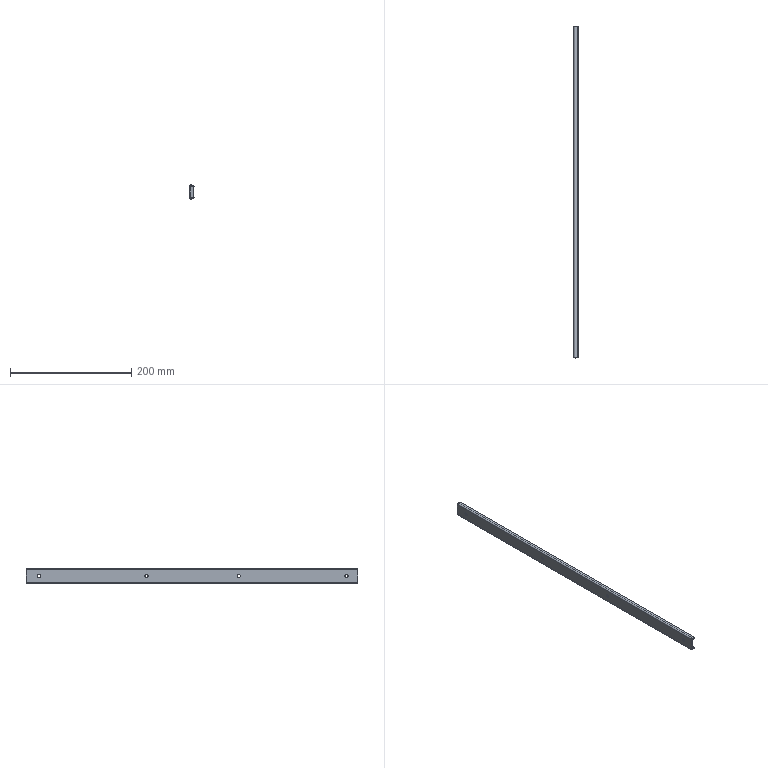Part | NX | features SLIDER_5003_009_C-SRH51Y22 2 | 1 solid | 39 faces | box 7 x 548.5 x 23.6 mm | volume 29924 mm3 | plane 20 | cylinder 19 | commonest cylinder face diameters 4.5 x8 0.4 x2 2 x2 3.6 x2 4.8 x2 8 x2
STEP:
#1=CARTESIAN_POINT('',(193.825,-253.,-88.75));
#2=VERTEX_POINT('',#1);
#3=CARTESIAN_POINT('',(193.825,-253.,-84.25));
#4=VERTEX_POINT('',#3);
#5=CARTESIAN_POINT('',(193.825,-253.,-86.5));
#6=DIRECTION('',(1.,0.,0.));
#7=DIRECTION('',(0.,0.,-1.));
#8=AXIS2_PLACEMENT_3D('',#5,#6,#7);
#9=CIRCLE('',#8,2.25);
#10=EDGE_CURVE('',#2,#4,#9,.F.);
#11=ORIENTED_EDGE('',*,*,#10,.F.);
#12=CARTESIAN_POINT('',(193.825,-252.2,-88.75));
#13=VERTEX_POINT('',#12);
#14=CARTESIAN_POINT('',(193.825,99.,-88.75));
#15=DIRECTION('',(0.,-1.,0.));
#16=VECTOR('',#15,1000.);
#17=LINE('',#14,#16);
#18=EDGE_CURVE('',#13,#2,#17,.T.);
#19=ORIENTED_EDGE('',*,*,#18,.F.);
#20=CARTESIAN_POINT('',(193.825,-252.2,-84.25));
#21=VERTEX_POINT('',#20);
#22=CARTESIAN_POINT('',(193.825,-252.2,-86.5));
#23=DIRECTION('',(1.,0.,0.));
#24=DIRECTION('',(0.,0.,-1.));
#25=AXIS2_PLACEMENT_3D('',#22,#23,#24);
#26=CIRCLE('',#25,2.25);
#27=EDGE_CURVE('',#21,#13,#26,.F.);
#28=ORIENTED_EDGE('',*,*,#27,.F.);
#29=CARTESIAN_POINT('',(193.825,99.,-84.25));
#30=DIRECTION('',(0.,1.,0.));
#31=VECTOR('',#30,1000.);
#32=LINE('',#29,#31);
#33=EDGE_CURVE('',#4,#21,#32,.T.);
#34=ORIENTED_EDGE('',*,*,#33,.F.);
#35=EDGE_LOOP('',(#11,#19,#28,#34));
#36=FACE_BOUND('',#35,.T.);
#37=CARTESIAN_POINT('',(193.825,-430.8,-88.75));
#38=VERTEX_POINT('',#37);
#39=CARTESIAN_POINT('',(193.825,-430.8,-84.25));
#40=VERTEX_POINT('',#39);
#41=CARTESIAN_POINT('',(193.825,-430.8,-86.5));
#42=DIRECTION('',(1.,0.,0.));
#43=DIRECTION('',(0.,0.,-1.));
#44=AXIS2_PLACEMENT_3D('',#41,#42,#43);
#45=CIRCLE('',#44,2.25);
#46=EDGE_CURVE('',#38,#40,#45,.F.);
#47=ORIENTED_EDGE('',*,*,#46,.F.);
#48=CARTESIAN_POINT('',(193.825,-430.,-88.75));
#49=VERTEX_POINT('',#48);
#50=CARTESIAN_POINT('',(193.825,99.,-88.75));
#51=DIRECTION('',(0.,-1.,0.));
#52=VECTOR('',#51,1000.);
#53=LINE('',#50,#52);
#54=EDGE_CURVE('',#49,#38,#53,.T.);
#55=ORIENTED_EDGE('',*,*,#54,.F.);
#56=CARTESIAN_POINT('',(193.825,-430.,-84.25));
#57=VERTEX_POINT('',#56);
#58=CARTESIAN_POINT('',(193.825,-430.,-86.5));
#59=DIRECTION('',(1.,0.,0.));
#60=DIRECTION('',(0.,0.,-1.));
#61=AXIS2_PLACEMENT_3D('',#58,#59,#60);
#62=CIRCLE('',#61,2.25);
#63=EDGE_CURVE('',#57,#49,#62,.F.);
#64=ORIENTED_EDGE('',*,*,#63,.F.);
#65=CARTESIAN_POINT('',(193.825,99.,-84.25));
#66=DIRECTION('',(0.,1.,0.));
#67=VECTOR('',#66,1000.);
#68=LINE('',#65,#67);
#69=EDGE_CURVE('',#40,#57,#68,.T.);
#70=ORIENTED_EDGE('',*,*,#69,.F.);
#71=EDGE_LOOP('',(#47,#55,#64,#70));
#72=FACE_BOUND('',#71,.T.);
#73=CARTESIAN_POINT('',(193.825,97.4,-77.5));
#74=VERTEX_POINT('',#73);
#75=CARTESIAN_POINT('',(193.825,97.4,-76.5));
#76=VERTEX_POINT('',#75);
#77=CARTESIAN_POINT('',(193.825,97.4,-98.3));
#78=DIRECTION('',(0.,0.,1.));
#79=VECTOR('',#78,1000.);
#80=LINE('',#77,#79);
#81=EDGE_CURVE('',#74,#76,#80,.T.);
#82=ORIENTED_EDGE('',*,*,#81,.F.);
#83=CARTESIAN_POINT('',(193.825,97.4,-95.5));
#84=VERTEX_POINT('',#83);
#85=CARTESIAN_POINT('',(193.825,97.4,-96.5));
#86=DIRECTION('',(0.,0.,1.));
#87=VECTOR('',#86,1000.);
#88=LINE('',#85,#87);
#89=EDGE_CURVE('',#74,#84,#88,.F.);
#90=ORIENTED_EDGE('',*,*,#89,.T.);
#91=CARTESIAN_POINT('',(193.825,97.4,-96.5));
#92=VERTEX_POINT('',#91);
#93=CARTESIAN_POINT('',(193.825,97.4,-98.3));
#94=DIRECTION('',(0.,0.,1.));
#95=VECTOR('',#94,1000.);
#96=LINE('',#93,#95);
#97=EDGE_CURVE('',#92,#84,#96,.T.);
#98=ORIENTED_EDGE('',*,*,#97,.F.);
#99=CARTESIAN_POINT('',(193.825,-449.5,-96.5));
#100=VERTEX_POINT('',#99);
#101=CARTESIAN_POINT('',(193.825,99.,-96.5));
#102=DIRECTION('',(0.,-1.,0.));
#103=VECTOR('',#102,1000.);
#104=LINE('',#101,#103);
#105=EDGE_CURVE('',#92,#100,#104,.T.);
#106=ORIENTED_EDGE('',*,*,#105,.T.);
#107=CARTESIAN_POINT('',(193.825,-449.5,-76.5));
#108=VERTEX_POINT('',#107);
#109=CARTESIAN_POINT('',(193.825,-449.5,-96.5));
#110=DIRECTION('',(0.,0.,1.));
#111=VECTOR('',#110,1000.);
#112=LINE('',#109,#111);
#113=EDGE_CURVE('',#100,#108,#112,.T.);
#114=ORIENTED_EDGE('',*,*,#113,.T.);
#115=CARTESIAN_POINT('',(193.825,99.,-76.5));
#116=DIRECTION('',(0.,-1.,0.));
#117=VECTOR('',#116,1000.);
#118=LINE('',#115,#117);
#119=EDGE_CURVE('',#76,#108,#118,.T.);
#120=ORIENTED_EDGE('',*,*,#119,.F.);
#121=EDGE_LOOP('',(#82,#90,#98,#106,#114,#120));
#122=FACE_BOUND('',#121,.T.);
#123=CARTESIAN_POINT('',(193.825,78.,-84.25));
#124=VERTEX_POINT('',#123);
#125=CARTESIAN_POINT('',(193.825,78.,-88.75));
#126=VERTEX_POINT('',#125);
#127=CARTESIAN_POINT('',(193.825,78.,-86.5));
#128=DIRECTION('',(1.,0.,0.));
#129=DIRECTION('',(0.,0.,-1.));
#130=AXIS2_PLACEMENT_3D('',#127,#128,#129);
#131=CIRCLE('',#130,2.25);
#132=EDGE_CURVE('',#124,#126,#131,.F.);
#133=ORIENTED_EDGE('',*,*,#132,.F.);
#134=CARTESIAN_POINT('',(193.825,77.2,-84.25));
#135=VERTEX_POINT('',#134);
#136=CARTESIAN_POINT('',(193.825,99.,-84.25));
#137=DIRECTION('',(0.,1.,0.));
#138=VECTOR('',#137,1000.);
#139=LINE('',#136,#138);
#140=EDGE_CURVE('',#135,#124,#139,.T.);
#141=ORIENTED_EDGE('',*,*,#140,.F.);
#142=CARTESIAN_POINT('',(193.825,77.2,-88.75));
#143=VERTEX_POINT('',#142);
#144=CARTESIAN_POINT('',(193.825,77.2,-86.5));
#145=DIRECTION('',(1.,0.,0.));
#146=DIRECTION('',(0.,0.,-1.));
#147=AXIS2_PLACEMENT_3D('',#144,#145,#146);
#148=CIRCLE('',#147,2.25);
#149=EDGE_CURVE('',#143,#135,#148,.F.);
#150=ORIENTED_EDGE('',*,*,#149,.F.);
#151=CARTESIAN_POINT('',(193.825,99.,-88.75));
#152=DIRECTION('',(0.,-1.,0.));
#153=VECTOR('',#152,1000.);
#154=LINE('',#151,#153);
#155=EDGE_CURVE('',#126,#143,#154,.T.);
#156=ORIENTED_EDGE('',*,*,#155,.F.);
#157=EDGE_LOOP('',(#133,#141,#150,#156));
#158=FACE_BOUND('',#157,.T.);
#159=CARTESIAN_POINT('',(193.825,-100.6,-88.75));
#160=VERTEX_POINT('',#159);
#161=CARTESIAN_POINT('',(193.825,-100.6,-84.25));
#162=VERTEX_POINT('',#161);
#163=CARTESIAN_POINT('',(193.825,-100.6,-86.5));
#164=DIRECTION('',(1.,0.,0.));
#165=DIRECTION('',(0.,0.,-1.));
#166=AXIS2_PLACEMENT_3D('',#163,#164,#165);
#167=CIRCLE('',#166,2.25);
#168=EDGE_CURVE('',#160,#162,#167,.F.);
#169=ORIENTED_EDGE('',*,*,#168,.F.);
#170=CARTESIAN_POINT('',(193.825,-99.8,-88.75));
#171=VERTEX_POINT('',#170);
#172=CARTESIAN_POINT('',(193.825,99.,-88.75));
#173=DIRECTION('',(0.,-1.,0.));
#174=VECTOR('',#173,1000.);
#175=LINE('',#172,#174);
#176=EDGE_CURVE('',#171,#160,#175,.T.);
#177=ORIENTED_EDGE('',*,*,#176,.F.);
#178=CARTESIAN_POINT('',(193.825,-99.8,-84.25));
#179=VERTEX_POINT('',#178);
#180=CARTESIAN_POINT('',(193.825,-99.8,-86.5));
#181=DIRECTION('',(1.,0.,0.));
#182=DIRECTION('',(0.,0.,-1.));
#183=AXIS2_PLACEMENT_3D('',#180,#181,#182);
#184=CIRCLE('',#183,2.25);
#185=EDGE_CURVE('',#179,#171,#184,.F.);
#186=ORIENTED_EDGE('',*,*,#185,.F.);
#187=CARTESIAN_POINT('',(193.825,99.,-84.25));
#188=DIRECTION('',(0.,1.,0.));
#189=VECTOR('',#188,1000.);
#190=LINE('',#187,#189);
#191=EDGE_CURVE('',#162,#179,#190,.T.);
#192=ORIENTED_EDGE('',*,*,#191,.F.);
#193=EDGE_LOOP('',(#169,#177,#186,#192));
#194=FACE_BOUND('',#193,.T.);
#195=CARTESIAN_POINT('',(193.825,99.,-96.5));
#196=DIRECTION('',(1.,0.,0.));
#197=DIRECTION('',(0.,0.,-1.));
#198=AXIS2_PLACEMENT_3D('',#195,#196,#197);
#199=PLANE('',#198);
#200=ADVANCED_FACE('',(#36,#72,#122,#158,#194),#199,.F.);
#201=CARTESIAN_POINT('',(195.425,-253.,-88.75));
#202=VERTEX_POINT('',#201);
#203=CARTESIAN_POINT('',(195.425,-253.,-84.25));
#204=VERTEX_POINT('',#203);
#205=CARTESIAN_POINT('',(195.425,-253.,-86.5));
#206=DIRECTION('',(-1.,0.,0.));
#207=DIRECTION('',(0.,1.,0.));
#208=AXIS2_PLACEMENT_3D('',#205,#206,#207);
#209=CIRCLE('',#208,2.25);
#210=EDGE_CURVE('',#202,#204,#209,.T.);
#211=ORIENTED_EDGE('',*,*,#210,.T.);
#212=CARTESIAN_POINT('',(195.425,-252.2,-84.25));
#213=VERTEX_POINT('',#212);
#214=CARTESIAN_POINT('',(195.425,-253.,-84.25));
#215=DIRECTION('',(0.,1.,0.));
#216=VECTOR('',#215,1000.);
#217=LINE('',#214,#216);
#218=EDGE_CURVE('',#204,#213,#217,.T.);
#219=ORIENTED_EDGE('',*,*,#218,.T.);
#220=CARTESIAN_POINT('',(195.425,-252.2,-88.75));
#221=VERTEX_POINT('',#220);
#222=CARTESIAN_POINT('',(195.425,-252.2,-86.5));
#223=DIRECTION('',(-1.,0.,0.));
#224=DIRECTION('',(0.,1.,0.));
#225=AXIS2_PLACEMENT_3D('',#222,#223,#224);
#226=CIRCLE('',#225,2.25);
#227=EDGE_CURVE('',#213,#221,#226,.T.);
#228=ORIENTED_EDGE('',*,*,#227,.T.);
#229=CARTESIAN_POINT('',(195.425,-253.,-88.75));
#230=DIRECTION('',(0.,-1.,0.));
#231=VECTOR('',#230,1000.);
#232=LINE('',#229,#231);
#233=EDGE_CURVE('',#221,#202,#232,.T.);
#234=ORIENTED_EDGE('',*,*,#233,.T.);
#235=EDGE_LOOP('',(#211,#219,#228,#234));
#236=FACE_BOUND('',#235,.T.);
#237=CARTESIAN_POINT('',(195.425,-430.8,-88.75));
#238=VERTEX_POINT('',#237);
#239=CARTESIAN_POINT('',(195.425,-430.8,-84.25));
#240=VERTEX_POINT('',#239);
#241=CARTESIAN_POINT('',(195.425,-430.8,-86.5));
#242=DIRECTION('',(-1.,0.,0.));
#243=DIRECTION('',(0.,1.,0.));
#244=AXIS2_PLACEMENT_3D('',#241,#242,#243);
#245=CIRCLE('',#244,2.25);
#246=EDGE_CURVE('',#238,#240,#245,.T.);
#247=ORIENTED_EDGE('',*,*,#246,.T.);
#248=CARTESIAN_POINT('',(195.425,-430.,-84.25));
#249=VERTEX_POINT('',#248);
#250=CARTESIAN_POINT('',(195.425,-430.8,-84.25));
#251=DIRECTION('',(0.,1.,0.));
#252=VECTOR('',#251,1000.);
#253=LINE('',#250,#252);
#254=EDGE_CURVE('',#240,#249,#253,.T.);
#255=ORIENTED_EDGE('',*,*,#254,.T.);
#256=CARTESIAN_POINT('',(195.425,-430.,-88.75));
#257=VERTEX_POINT('',#256);
#258=CARTESIAN_POINT('',(195.425,-430.,-86.5));
#259=DIRECTION('',(-1.,0.,0.));
#260=DIRECTION('',(0.,1.,0.));
#261=AXIS2_PLACEMENT_3D('',#258,#259,#260);
#262=CIRCLE('',#261,2.25);
#263=EDGE_CURVE('',#249,#257,#262,.T.);
#264=ORIENTED_EDGE('',*,*,#263,.T.);
#265=CARTESIAN_POINT('',(195.425,-430.8,-88.75));
#266=DIRECTION('',(0.,-1.,0.));
#267=VECTOR('',#266,1000.);
#268=LINE('',#265,#267);
#269=EDGE_CURVE('',#257,#238,#268,.T.);
#270=ORIENTED_EDGE('',*,*,#269,.T.);
#271=EDGE_LOOP('',(#247,#255,#264,#270));
#272=FACE_BOUND('',#271,.T.);
#273=CARTESIAN_POINT('',(195.425,97.4,-96.5));
#274=VERTEX_POINT('',#273);
#275=CARTESIAN_POINT('',(195.425,-449.5,-96.5));
#276=VERTEX_POINT('',#275);
#277=CARTESIAN_POINT('',(195.425,99.,-96.5));
#278=DIRECTION('',(0.,-1.,0.));
#279=VECTOR('',#278,1000.);
#280=LINE('',#277,#279);
#281=EDGE_CURVE('',#274,#276,#280,.T.);
#282=ORIENTED_EDGE('',*,*,#281,.F.);
#283=CARTESIAN_POINT('',(195.425,97.4,-95.5));
#284=VERTEX_POINT('',#283);
#285=CARTESIAN_POINT('',(195.425,97.4,-96.5));
#286=DIRECTION('',(0.,0.,1.));
#287=VECTOR('',#286,1000.);
#288=LINE('',#285,#287);
#289=EDGE_CURVE('',#274,#284,#288,.T.);
#290=ORIENTED_EDGE('',*,*,#289,.T.);
#291=CARTESIAN_POINT('',(195.425,97.4,-77.5));
#292=VERTEX_POINT('',#291);
#293=CARTESIAN_POINT('',(195.425,97.4,-96.5));
#294=DIRECTION('',(0.,0.,1.));
#295=VECTOR('',#294,1000.);
#296=LINE('',#293,#295);
#297=EDGE_CURVE('',#284,#292,#296,.T.);
#298=ORIENTED_EDGE('',*,*,#297,.T.);
#299=CARTESIAN_POINT('',(195.425,97.4,-76.5));
#300=VERTEX_POINT('',#299);
#301=CARTESIAN_POINT('',(195.425,97.4,-96.5));
#302=DIRECTION('',(0.,0.,1.));
#303=VECTOR('',#302,1000.);
#304=LINE('',#301,#303);
#305=EDGE_CURVE('',#292,#300,#304,.T.);
#306=ORIENTED_EDGE('',*,*,#305,.T.);
#307=CARTESIAN_POINT('',(195.425,-449.5,-76.5));
#308=VERTEX_POINT('',#307);
#309=CARTESIAN_POINT('',(195.425,99.,-76.5));
#310=DIRECTION('',(0.,-1.,0.));
#311=VECTOR('',#310,1000.);
#312=LINE('',#309,#311);
#313=EDGE_CURVE('',#300,#308,#312,.T.);
#314=ORIENTED_EDGE('',*,*,#313,.T.);
#315=CARTESIAN_POINT('',(195.425,-449.5,-96.5));
#316=DIRECTION('',(0.,0.,-1.));
#317=VECTOR('',#316,1000.);
#318=LINE('',#315,#317);
#319=EDGE_CURVE('',#308,#276,#318,.T.);
#320=ORIENTED_EDGE('',*,*,#319,.T.);
#321=EDGE_LOOP('',(#282,#290,#298,#306,#314,#320));
#322=FACE_BOUND('',#321,.T.);
#323=CARTESIAN_POINT('',(195.425,78.,-84.25));
#324=VERTEX_POINT('',#323);
#325=CARTESIAN_POINT('',(195.425,78.,-88.75));
#326=VERTEX_POINT('',#325);
#327=CARTESIAN_POINT('',(195.425,78.,-86.5));
#328=DIRECTION('',(-1.,0.,0.));
#329=DIRECTION('',(0.,1.,0.));
#330=AXIS2_PLACEMENT_3D('',#327,#328,#329);
#331=CIRCLE('',#330,2.25);
#332=EDGE_CURVE('',#324,#326,#331,.T.);
#333=ORIENTED_EDGE('',*,*,#332,.T.);
#334=CARTESIAN_POINT('',(195.425,77.2,-88.75));
#335=VERTEX_POINT('',#334);
#336=CARTESIAN_POINT('',(195.425,77.2,-88.75));
#337=DIRECTION('',(0.,-1.,0.));
#338=VECTOR('',#337,1000.);
#339=LINE('',#336,#338);
#340=EDGE_CURVE('',#326,#335,#339,.T.);
#341=ORIENTED_EDGE('',*,*,#340,.T.);
#342=CARTESIAN_POINT('',(195.425,77.2,-84.25));
#343=VERTEX_POINT('',#342);
#344=CARTESIAN_POINT('',(195.425,77.2,-86.5));
#345=DIRECTION('',(-1.,0.,0.));
#346=DIRECTION('',(0.,1.,0.));
#347=AXIS2_PLACEMENT_3D('',#344,#345,#346);
#348=CIRCLE('',#347,2.25);
#349=EDGE_CURVE('',#335,#343,#348,.T.);
#350=ORIENTED_EDGE('',*,*,#349,.T.);
#351=CARTESIAN_POINT('',(195.425,77.2,-84.25));
#352=DIRECTION('',(0.,1.,0.));
#353=VECTOR('',#352,1000.);
#354=LINE('',#351,#353);
#355=EDGE_CURVE('',#343,#324,#354,.T.);
#356=ORIENTED_EDGE('',*,*,#355,.T.);
#357=EDGE_LOOP('',(#333,#341,#350,#356));
#358=FACE_BOUND('',#357,.T.);
#359=CARTESIAN_POINT('',(195.425,-100.6,-88.75));
#360=VERTEX_POINT('',#359);
#361=CARTESIAN_POINT('',(195.425,-100.6,-84.25));
#362=VERTEX_POINT('',#361);
#363=CARTESIAN_POINT('',(195.425,-100.6,-86.5));
#364=DIRECTION('',(-1.,0.,0.));
#365=DIRECTION('',(0.,1.,0.));
#366=AXIS2_PLACEMENT_3D('',#363,#364,#365);
#367=CIRCLE('',#366,2.25);
#368=EDGE_CURVE('',#360,#362,#367,.T.);
#369=ORIENTED_EDGE('',*,*,#368,.T.);
#370=CARTESIAN_POINT('',(195.425,-99.8,-84.25));
#371=VERTEX_POINT('',#370);
#372=CARTESIAN_POINT('',(195.425,-100.6,-84.25));
#373=DIRECTION('',(0.,1.,0.));
#374=VECTOR('',#373,1000.);
#375=LINE('',#372,#374);
#376=EDGE_CURVE('',#362,#371,#375,.T.);
#377=ORIENTED_EDGE('',*,*,#376,.T.);
#378=CARTESIAN_POINT('',(195.425,-99.8,-88.75));
#379=VERTEX_POINT('',#378);
#380=CARTESIAN_POINT('',(195.425,-99.8,-86.5));
#381=DIRECTION('',(-1.,0.,0.));
#382=DIRECTION('',(0.,1.,0.));
#383=AXIS2_PLACEMENT_3D('',#380,#381,#382);
#384=CIRCLE('',#383,2.25);
#385=EDGE_CURVE('',#371,#379,#384,.T.);
#386=ORIENTED_EDGE('',*,*,#385,.T.);
#387=CARTESIAN_POINT('',(195.425,-100.6,-88.75));
#388=DIRECTION('',(0.,-1.,0.));
#389=VECTOR('',#388,1000.);
#390=LINE('',#387,#389);
#391=EDGE_CURVE('',#379,#360,#390,.T.);
#392=ORIENTED_EDGE('',*,*,#391,.T.);
#393=EDGE_LOOP('',(#369,#377,#386,#392));
#394=FACE_BOUND('',#393,.T.);
#395=CARTESIAN_POINT('',(195.425,99.,-96.5));
#396=DIRECTION('',(-1.,0.,0.));
#397=DIRECTION('',(0.,0.,1.));
#398=AXIS2_PLACEMENT_3D('',#395,#396,#397);
#399=PLANE('',#398);
#400=ADVANCED_FACE('',(#236,#272,#322,#358,#394),#399,.F.);
#401=CARTESIAN_POINT('',(198.325,97.4,-95.5));
#402=VERTEX_POINT('',#401);
#403=CARTESIAN_POINT('',(197.931,97.4,-95.5));
#404=VERTEX_POINT('',#403);
#405=CARTESIAN_POINT('',(199.325,97.4,-95.5));
#406=DIRECTION('',(-1.,0.,0.));
#407=VECTOR('',#406,1000.);
#408=LINE('',#405,#407);
#409=EDGE_CURVE('',#402,#404,#408,.T.);
#410=ORIENTED_EDGE('',*,*,#409,.F.);
#411=CARTESIAN_POINT('',(198.667,97.4,-95.44));
#412=VERTEX_POINT('',#411);
#413=CARTESIAN_POINT('',(198.325,97.4,-94.5));
#414=DIRECTION('',(0.,-1.,0.));
#415=DIRECTION('',(-1.,0.,0.));
#416=AXIS2_PLACEMENT_3D('',#413,#414,#415);
#417=CIRCLE('',#416,1.);
#418=EDGE_CURVE('',#402,#412,#417,.T.);
#419=ORIENTED_EDGE('',*,*,#418,.T.);
#420=CARTESIAN_POINT('',(200.825,97.4,-96.099));
#421=VERTEX_POINT('',#420);
#422=CARTESIAN_POINT('',(198.625,97.4,-99.439));
#423=DIRECTION('',(0.,-1.,0.));
#424=DIRECTION('',(-1.,0.,0.));
#425=AXIS2_PLACEMENT_3D('',#422,#423,#424);
#426=CIRCLE('',#425,4.);
#427=EDGE_CURVE('',#421,#412,#426,.T.);
#428=ORIENTED_EDGE('',*,*,#427,.F.);
#429=CARTESIAN_POINT('',(200.425,97.4,-97.852));
#430=VERTEX_POINT('',#429);
#431=CARTESIAN_POINT('',(200.425,97.4,-97.852));
#432=DIRECTION('',(0.2224,0.,0.9749));
#433=VECTOR('',#432,1000.);
#434=LINE('',#431,#433);
#435=EDGE_CURVE('',#430,#421,#434,.T.);
#436=ORIENTED_EDGE('',*,*,#435,.F.);
#437=CARTESIAN_POINT('',(196.911,97.4,-97.76));
#438=VERTEX_POINT('',#437);
#439=CARTESIAN_POINT('',(198.625,97.4,-99.439));
#440=DIRECTION('',(0.,-1.,0.));
#441=DIRECTION('',(-1.,0.,0.));
#442=AXIS2_PLACEMENT_3D('',#439,#440,#441);
#443=CIRCLE('',#442,2.4);
#444=EDGE_CURVE('',#438,#430,#443,.F.);
#445=ORIENTED_EDGE('',*,*,#444,.F.);
#446=CARTESIAN_POINT('',(195.625,97.4,-96.5));
#447=DIRECTION('',(0.,-1.,0.));
#448=DIRECTION('',(-1.,0.,0.));
#449=AXIS2_PLACEMENT_3D('',#446,#447,#448);
#450=CIRCLE('',#449,1.8);
#451=EDGE_CURVE('',#92,#438,#450,.T.);
#452=ORIENTED_EDGE('',*,*,#451,.F.);
#453=ORIENTED_EDGE('',*,*,#97,.T.);
#454=CARTESIAN_POINT('',(199.325,97.4,-95.5));
#455=DIRECTION('',(-1.,0.,0.));
#456=VECTOR('',#455,1000.);
#457=LINE('',#454,#456);
#458=EDGE_CURVE('',#284,#84,#457,.T.);
#459=ORIENTED_EDGE('',*,*,#458,.F.);
#460=ORIENTED_EDGE('',*,*,#289,.F.);
#461=CARTESIAN_POINT('',(195.768,97.4,-96.64));
#462=VERTEX_POINT('',#461);
#463=CARTESIAN_POINT('',(195.625,97.4,-96.5));
#464=DIRECTION('',(0.,-1.,0.));
#465=DIRECTION('',(-1.,0.,0.));
#466=AXIS2_PLACEMENT_3D('',#463,#464,#465);
#467=CIRCLE('',#466,0.2);
#468=EDGE_CURVE('',#462,#274,#467,.F.);
#469=ORIENTED_EDGE('',*,*,#468,.F.);
#470=CARTESIAN_POINT('',(198.625,97.4,-99.439));
#471=DIRECTION('',(0.,-1.,0.));
#472=DIRECTION('',(-1.,0.,0.));
#473=AXIS2_PLACEMENT_3D('',#470,#471,#472);
#474=CIRCLE('',#473,4.);
#475=EDGE_CURVE('',#404,#462,#474,.T.);
#476=ORIENTED_EDGE('',*,*,#475,.F.);
#477=EDGE_LOOP('',(#410,#419,#428,#436,#445,#452,#453,#459,#460,#469,#476));
#478=FACE_BOUND('',#477,.T.);
#479=CARTESIAN_POINT('',(200.825,97.4,-98.3));
#480=DIRECTION('',(0.,-1.,0.));
#481=DIRECTION('',(-1.,0.,0.));
#482=AXIS2_PLACEMENT_3D('',#479,#480,#481);
#483=PLANE('',#482);
#484=ADVANCED_FACE('',(#478),#483,.F.);
#485=ORIENTED_EDGE('',*,*,#105,.F.);
#486=ORIENTED_EDGE('',*,*,#451,.T.);
#487=CARTESIAN_POINT('',(196.911,-449.5,-97.76));
#488=VERTEX_POINT('',#487);
#489=CARTESIAN_POINT('',(196.911,99.,-97.76));
#490=DIRECTION('',(0.,-1.,0.));
#491=VECTOR('',#490,1000.);
#492=LINE('',#489,#491);
#493=EDGE_CURVE('',#438,#488,#492,.T.);
#494=ORIENTED_EDGE('',*,*,#493,.T.);
#495=CARTESIAN_POINT('',(195.625,-449.5,-96.5));
#496=DIRECTION('',(0.,1.,0.));
#497=DIRECTION('',(-1.,0.,0.));
#498=AXIS2_PLACEMENT_3D('',#495,#496,#497);
#499=CIRCLE('',#498,1.8);
#500=EDGE_CURVE('',#488,#100,#499,.T.);
#501=ORIENTED_EDGE('',*,*,#500,.T.);
#502=EDGE_LOOP('',(#485,#486,#494,#501));
#503=FACE_BOUND('',#502,.T.);
#504=CARTESIAN_POINT('',(195.625,99.,-96.5));
#505=DIRECTION('',(0.,-1.,0.));
#506=DIRECTION('',(-1.,0.,0.));
#507=AXIS2_PLACEMENT_3D('',#504,#505,#506);
#508=CYLINDRICAL_SURFACE('',#507,1.8);
#509=ADVANCED_FACE('',(#503),#508,.T.);
#510=CARTESIAN_POINT('',(196.911,97.4,-75.24));
#511=VERTEX_POINT('',#510);
#512=CARTESIAN_POINT('',(196.911,-449.5,-75.24));
#513=VERTEX_POINT('',#512);
#514=CARTESIAN_POINT('',(196.911,99.,-75.24));
#515=DIRECTION('',(0.,-1.,0.));
#516=VECTOR('',#515,1000.);
#517=LINE('',#514,#516);
#518=EDGE_CURVE('',#511,#513,#517,.T.);
#519=ORIENTED_EDGE('',*,*,#518,.F.);
#520=CARTESIAN_POINT('',(195.625,97.4,-76.5));
#521=DIRECTION('',(0.,-1.,0.));
#522=DIRECTION('',(-1.,0.,0.));
#523=AXIS2_PLACEMENT_3D('',#520,#521,#522);
#524=CIRCLE('',#523,1.8);
#525=EDGE_CURVE('',#511,#76,#524,.T.);
#526=ORIENTED_EDGE('',*,*,#525,.T.);
#527=ORIENTED_EDGE('',*,*,#119,.T.);
#528=CARTESIAN_POINT('',(195.625,-449.5,-76.5));
#529=DIRECTION('',(0.,1.,0.));
#530=DIRECTION('',(1.,0.,0.));
#531=AXIS2_PLACEMENT_3D('',#528,#529,#530);
#532=CIRCLE('',#531,1.8);
#533=EDGE_CURVE('',#108,#513,#532,.T.);
#534=ORIENTED_EDGE('',*,*,#533,.T.);
#535=EDGE_LOOP('',(#519,#526,#527,#534));
#536=FACE_BOUND('',#535,.T.);
#537=CARTESIAN_POINT('',(195.625,99.,-76.5));
#538=DIRECTION('',(0.,-1.,0.));
#539=DIRECTION('',(-1.,0.,0.));
#540=AXIS2_PLACEMENT_3D('',#537,#538,#539);
#541=CYLINDRICAL_SURFACE('',#540,1.8);
#542=ADVANCED_FACE('',(#536),#541,.T.);
#543=CARTESIAN_POINT('',(200.425,97.4,-75.148));
#544=VERTEX_POINT('',#543);
#545=CARTESIAN_POINT('',(200.425,-449.5,-75.148));
#546=VERTEX_POINT('',#545);
#547=CARTESIAN_POINT('',(200.425,99.,-75.148));
#548=DIRECTION('',(0.,-1.,0.));
#549=VECTOR('',#548,1000.);
#550=LINE('',#547,#549);
#551=EDGE_CURVE('',#544,#546,#550,.T.);
#552=ORIENTED_EDGE('',*,*,#551,.F.);
#553=CARTESIAN_POINT('',(198.625,97.4,-73.561));
#554=DIRECTION('',(0.,-1.,0.));
#555=DIRECTION('',(-1.,0.,0.));
#556=AXIS2_PLACEMENT_3D('',#553,#554,#555);
#557=CIRCLE('',#556,2.4);
#558=EDGE_CURVE('',#544,#511,#557,.F.);
#559=ORIENTED_EDGE('',*,*,#558,.T.);
#560=ORIENTED_EDGE('',*,*,#518,.T.);
#561=CARTESIAN_POINT('',(198.625,-449.5,-73.561));
#562=DIRECTION('',(0.,-1.,0.));
#563=DIRECTION('',(-1.,0.,0.));
#564=AXIS2_PLACEMENT_3D('',#561,#562,#563);
#565=CIRCLE('',#564,2.4);
#566=EDGE_CURVE('',#513,#546,#565,.T.);
#567=ORIENTED_EDGE('',*,*,#566,.T.);
#568=EDGE_LOOP('',(#552,#559,#560,#567));
#569=FACE_BOUND('',#568,.T.);
#570=CARTESIAN_POINT('',(198.625,99.,-73.561));
#571=DIRECTION('',(0.,-1.,0.));
#572=DIRECTION('',(-1.,0.,0.));
#573=AXIS2_PLACEMENT_3D('',#570,#571,#572);
#574=CYLINDRICAL_SURFACE('',#573,2.4);
#575=ADVANCED_FACE('',(#569),#574,.F.);
#576=CARTESIAN_POINT('',(200.825,97.4,-76.901));
#577=VERTEX_POINT('',#576);
#578=CARTESIAN_POINT('',(200.825,-449.5,-76.901));
#579=VERTEX_POINT('',#578);
#580=CARTESIAN_POINT('',(200.825,99.,-76.901));
#581=DIRECTION('',(0.,-1.,0.));
#582=VECTOR('',#581,1000.);
#583=LINE('',#580,#582);
#584=EDGE_CURVE('',#577,#579,#583,.T.);
#585=ORIENTED_EDGE('',*,*,#584,.F.);
#586=CARTESIAN_POINT('',(200.425,97.4,-75.148));
#587=DIRECTION('',(-0.2224,0.,0.9749));
#588=VECTOR('',#587,1000.);
#589=LINE('',#586,#588);
#590=EDGE_CURVE('',#577,#544,#589,.T.);
#591=ORIENTED_EDGE('',*,*,#590,.T.);
#592=ORIENTED_EDGE('',*,*,#551,.T.);
#593=CARTESIAN_POINT('',(200.425,-449.5,-75.148));
#594=DIRECTION('',(0.2224,0.,-0.9749));
#595=VECTOR('',#594,1000.);
#596=LINE('',#593,#595);
#597=EDGE_CURVE('',#546,#579,#596,.T.);
#598=ORIENTED_EDGE('',*,*,#597,.T.);
#599=EDGE_LOOP('',(#585,#591,#592,#598));
#600=FACE_BOUND('',#599,.T.);
#601=CARTESIAN_POINT('',(200.425,99.,-75.148));
#602=DIRECTION('',(-0.9749,0.,-0.2224));
#603=DIRECTION('',(-0.2224,0.,0.9749));
#604=AXIS2_PLACEMENT_3D('',#601,#602,#603);
#605=PLANE('',#604);
#606=ADVANCED_FACE('',(#600),#605,.F.);
#607=CARTESIAN_POINT('',(195.768,97.4,-76.36));
#608=VERTEX_POINT('',#607);
#609=CARTESIAN_POINT('',(195.768,-449.5,-76.36));
#610=VERTEX_POINT('',#609);
#611=CARTESIAN_POINT('',(195.768,99.,-76.36));
#612=DIRECTION('',(0.,-1.,0.));
#613=VECTOR('',#612,1000.);
#614=LINE('',#611,#613);
#615=EDGE_CURVE('',#608,#610,#614,.T.);
#616=ORIENTED_EDGE('',*,*,#615,.F.);
#617=CARTESIAN_POINT('',(197.931,97.4,-77.5));
#618=VERTEX_POINT('',#617);
#619=CARTESIAN_POINT('',(198.625,97.4,-73.561));
#620=DIRECTION('',(0.,-1.,0.));
#621=DIRECTION('',(-1.,0.,0.));
#622=AXIS2_PLACEMENT_3D('',#619,#620,#621);
#623=CIRCLE('',#622,4.);
#624=EDGE_CURVE('',#608,#618,#623,.T.);
#625=ORIENTED_EDGE('',*,*,#624,.T.);
#626=CARTESIAN_POINT('',(198.667,97.4,-77.56));
#627=VERTEX_POINT('',#626);
#628=CARTESIAN_POINT('',(198.625,97.4,-73.561));
#629=DIRECTION('',(0.,-1.,0.));
#630=DIRECTION('',(-1.,0.,0.));
#631=AXIS2_PLACEMENT_3D('',#628,#629,#630);
#632=CIRCLE('',#631,4.);
#633=EDGE_CURVE('',#618,#627,#632,.T.);
#634=ORIENTED_EDGE('',*,*,#633,.T.);
#635=CARTESIAN_POINT('',(198.625,97.4,-73.561));
#636=DIRECTION('',(0.,-1.,0.));
#637=DIRECTION('',(-1.,0.,0.));
#638=AXIS2_PLACEMENT_3D('',#635,#636,#637);
#639=CIRCLE('',#638,4.);
#640=EDGE_CURVE('',#627,#577,#639,.T.);
#641=ORIENTED_EDGE('',*,*,#640,.T.);
#642=ORIENTED_EDGE('',*,*,#584,.T.);
#643=CARTESIAN_POINT('',(198.625,-449.5,-73.561));
#644=DIRECTION('',(0.,1.,0.));
#645=DIRECTION('',(1.,0.,0.));
#646=AXIS2_PLACEMENT_3D('',#643,#644,#645);
#647=CIRCLE('',#646,4.);
#648=EDGE_CURVE('',#579,#610,#647,.T.);
#649=ORIENTED_EDGE('',*,*,#648,.T.);
#650=EDGE_LOOP('',(#616,#625,#634,#641,#642,#649));
#651=FACE_BOUND('',#650,.T.);
#652=CARTESIAN_POINT('',(198.625,99.,-73.561));
#653=DIRECTION('',(0.,-1.,0.));
#654=DIRECTION('',(-1.,0.,0.));
#655=AXIS2_PLACEMENT_3D('',#652,#653,#654);
#656=CYLINDRICAL_SURFACE('',#655,4.);
#657=ADVANCED_FACE('',(#651),#656,.T.);
#658=ORIENTED_EDGE('',*,*,#313,.F.);
#659=CARTESIAN_POINT('',(195.625,97.4,-76.5));
#660=DIRECTION('',(0.,-1.,0.));
#661=DIRECTION('',(-1.,0.,0.));
#662=AXIS2_PLACEMENT_3D('',#659,#660,#661);
#663=CIRCLE('',#662,0.2);
#664=EDGE_CURVE('',#300,#608,#663,.F.);
#665=ORIENTED_EDGE('',*,*,#664,.T.);
#666=ORIENTED_EDGE('',*,*,#615,.T.);
#667=CARTESIAN_POINT('',(195.625,-449.5,-76.5));
#668=DIRECTION('',(0.,-1.,0.));
#669=DIRECTION('',(-1.,0.,0.));
#670=AXIS2_PLACEMENT_3D('',#667,#668,#669);
#671=CIRCLE('',#670,0.2);
#672=EDGE_CURVE('',#610,#308,#671,.T.);
#673=ORIENTED_EDGE('',*,*,#672,.T.);
#674=EDGE_LOOP('',(#658,#665,#666,#673));
#675=FACE_BOUND('',#674,.T.);
#676=CARTESIAN_POINT('',(195.625,99.,-76.5));
#677=DIRECTION('',(0.,-1.,0.));
#678=DIRECTION('',(-1.,0.,0.));
#679=AXIS2_PLACEMENT_3D('',#676,#677,#678);
#680=CYLINDRICAL_SURFACE('',#679,0.2);
#681=ADVANCED_FACE('',(#675),#680,.F.);
#682=CARTESIAN_POINT('',(195.768,-449.5,-96.64));
#683=VERTEX_POINT('',#682);
#684=CARTESIAN_POINT('',(195.768,99.,-96.64));
#685=DIRECTION('',(0.,-1.,0.));
#686=VECTOR('',#685,1000.);
#687=LINE('',#684,#686);
#688=EDGE_CURVE('',#462,#683,#687,.T.);
#689=ORIENTED_EDGE('',*,*,#688,.F.);
#690=ORIENTED_EDGE('',*,*,#468,.T.);
#691=ORIENTED_EDGE('',*,*,#281,.T.);
#692=CARTESIAN_POINT('',(195.625,-449.5,-96.5));
#693=DIRECTION('',(0.,-1.,0.));
#694=DIRECTION('',(1.,0.,0.));
#695=AXIS2_PLACEMENT_3D('',#692,#693,#694);
#696=CIRCLE('',#695,0.2);
#697=EDGE_CURVE('',#276,#683,#696,.T.);
#698=ORIENTED_EDGE('',*,*,#697,.T.);
#699=EDGE_LOOP('',(#689,#690,#691,#698));
#700=FACE_BOUND('',#699,.T.);
#701=CARTESIAN_POINT('',(195.625,99.,-96.5));
#702=DIRECTION('',(0.,-1.,0.));
#703=DIRECTION('',(-1.,0.,0.));
#704=AXIS2_PLACEMENT_3D('',#701,#702,#703);
#705=CYLINDRICAL_SURFACE('',#704,0.2);
#706=ADVANCED_FACE('',(#700),#705,.F.);
#707=CARTESIAN_POINT('',(200.825,-449.5,-96.099));
#708=VERTEX_POINT('',#707);
#709=CARTESIAN_POINT('',(200.825,99.,-96.099));
#710=DIRECTION('',(0.,-1.,0.));
#711=VECTOR('',#710,1000.);
#712=LINE('',#709,#711);
#713=EDGE_CURVE('',#421,#708,#712,.T.);
#714=ORIENTED_EDGE('',*,*,#713,.F.);
#715=ORIENTED_EDGE('',*,*,#427,.T.);
#716=CARTESIAN_POINT('',(198.625,97.4,-99.439));
#717=DIRECTION('',(0.,-1.,0.));
#718=DIRECTION('',(-1.,0.,0.));
#719=AXIS2_PLACEMENT_3D('',#716,#717,#718);
#720=CIRCLE('',#719,4.);
#721=EDGE_CURVE('',#412,#404,#720,.T.);
#722=ORIENTED_EDGE('',*,*,#721,.T.);
#723=ORIENTED_EDGE('',*,*,#475,.T.);
#724=ORIENTED_EDGE('',*,*,#688,.T.);
#725=CARTESIAN_POINT('',(198.625,-449.5,-99.439));
#726=DIRECTION('',(0.,1.,0.));
#727=DIRECTION('',(-1.,0.,0.));
#728=AXIS2_PLACEMENT_3D('',#725,#726,#727);
#729=CIRCLE('',#728,4.);
#730=EDGE_CURVE('',#683,#708,#729,.T.);
#731=ORIENTED_EDGE('',*,*,#730,.T.);
#732=EDGE_LOOP('',(#714,#715,#722,#723,#724,#731));
#733=FACE_BOUND('',#732,.T.);
#734=CARTESIAN_POINT('',(198.625,99.,-99.439));
#735=DIRECTION('',(0.,-1.,0.));
#736=DIRECTION('',(-1.,0.,0.));
#737=AXIS2_PLACEMENT_3D('',#734,#735,#736);
#738=CYLINDRICAL_SURFACE('',#737,4.);
#739=ADVANCED_FACE('',(#733),#738,.T.);
#740=CARTESIAN_POINT('',(200.425,-449.5,-97.852));
#741=VERTEX_POINT('',#740);
#742=CARTESIAN_POINT('',(200.425,99.,-97.852));
#743=DIRECTION('',(0.,-1.,0.));
#744=VECTOR('',#743,1000.);
#745=LINE('',#742,#744);
#746=EDGE_CURVE('',#430,#741,#745,.T.);
#747=ORIENTED_EDGE('',*,*,#746,.F.);
#748=ORIENTED_EDGE('',*,*,#435,.T.);
#749=ORIENTED_EDGE('',*,*,#713,.T.);
#750=CARTESIAN_POINT('',(200.425,-449.5,-97.852));
#751=DIRECTION('',(-0.2224,0.,-0.9749));
#752=VECTOR('',#751,1000.);
#753=LINE('',#750,#752);
#754=EDGE_CURVE('',#708,#741,#753,.T.);
#755=ORIENTED_EDGE('',*,*,#754,.T.);
#756=EDGE_LOOP('',(#747,#748,#749,#755));
#757=FACE_BOUND('',#756,.T.);
#758=CARTESIAN_POINT('',(200.425,99.,-97.852));
#759=DIRECTION('',(-0.9749,0.,0.2224));
#760=DIRECTION('',(0.2224,0.,0.9749));
#761=AXIS2_PLACEMENT_3D('',#758,#759,#760);
#762=PLANE('',#761);
#763=ADVANCED_FACE('',(#757),#762,.F.);
#764=ORIENTED_EDGE('',*,*,#493,.F.);
#765=ORIENTED_EDGE('',*,*,#444,.T.);
#766=ORIENTED_EDGE('',*,*,#746,.T.);
#767=CARTESIAN_POINT('',(198.625,-449.5,-99.439));
#768=DIRECTION('',(0.,-1.,0.));
#769=DIRECTION('',(1.,0.,0.));
#770=AXIS2_PLACEMENT_3D('',#767,#768,#769);
#771=CIRCLE('',#770,2.4);
#772=EDGE_CURVE('',#741,#488,#771,.T.);
#773=ORIENTED_EDGE('',*,*,#772,.T.);
#774=EDGE_LOOP('',(#764,#765,#766,#773));
#775=FACE_BOUND('',#774,.T.);
#776=CARTESIAN_POINT('',(198.625,99.,-99.439));
#777=DIRECTION('',(0.,-1.,0.));
#778=DIRECTION('',(-1.,0.,0.));
#779=AXIS2_PLACEMENT_3D('',#776,#777,#778);
#780=CYLINDRICAL_SURFACE('',#779,2.4);
#781=ADVANCED_FACE('',(#775),#780,.F.);
#782=ORIENTED_EDGE('',*,*,#500,.F.);
#783=ORIENTED_EDGE('',*,*,#772,.F.);
#784=ORIENTED_EDGE('',*,*,#754,.F.);
#785=ORIENTED_EDGE('',*,*,#730,.F.);
#786=ORIENTED_EDGE('',*,*,#697,.F.);
#787=ORIENTED_EDGE('',*,*,#319,.F.);
#788=ORIENTED_EDGE('',*,*,#672,.F.);
#789=ORIENTED_EDGE('',*,*,#648,.F.);
#790=ORIENTED_EDGE('',*,*,#597,.F.);
#791=ORIENTED_EDGE('',*,*,#566,.F.);
#792=ORIENTED_EDGE('',*,*,#533,.F.);
#793=ORIENTED_EDGE('',*,*,#113,.F.);
#794=EDGE_LOOP('',(#782,#783,#784,#785,#786,#787,#788,#789,#790,#791,#792,#793));
#795=FACE_BOUND('',#794,.T.);
#796=CARTESIAN_POINT('',(195.625,-449.5,-96.5));
#797=DIRECTION('',(0.,-1.,0.));
#798=DIRECTION('',(-1.,0.,0.));
#799=AXIS2_PLACEMENT_3D('',#796,#797,#798);
#800=PLANE('',#799);
#801=ADVANCED_FACE('',(#795),#800,.T.);
#802=ORIENTED_EDGE('',*,*,#640,.F.);
#803=CARTESIAN_POINT('',(198.325,97.4,-77.5));
#804=VERTEX_POINT('',#803);
#805=CARTESIAN_POINT('',(198.325,97.4,-78.5));
#806=DIRECTION('',(0.,-1.,0.));
#807=DIRECTION('',(-1.,0.,0.));
#808=AXIS2_PLACEMENT_3D('',#805,#806,#807);
#809=CIRCLE('',#808,1.);
#810=EDGE_CURVE('',#627,#804,#809,.T.);
#811=ORIENTED_EDGE('',*,*,#810,.T.);
#812=CARTESIAN_POINT('',(199.325,97.4,-77.5));
#813=DIRECTION('',(-1.,0.,0.));
#814=VECTOR('',#813,1000.);
#815=LINE('',#812,#814);
#816=EDGE_CURVE('',#804,#618,#815,.T.);
#817=ORIENTED_EDGE('',*,*,#816,.T.);
#818=ORIENTED_EDGE('',*,*,#624,.F.);
#819=ORIENTED_EDGE('',*,*,#664,.F.);
#820=ORIENTED_EDGE('',*,*,#305,.F.);
#821=CARTESIAN_POINT('',(199.325,97.4,-77.5));
#822=DIRECTION('',(-1.,0.,0.));
#823=VECTOR('',#822,1000.);
#824=LINE('',#821,#823);
#825=EDGE_CURVE('',#292,#74,#824,.T.);
#826=ORIENTED_EDGE('',*,*,#825,.T.);
#827=ORIENTED_EDGE('',*,*,#81,.T.);
#828=ORIENTED_EDGE('',*,*,#525,.F.);
#829=ORIENTED_EDGE('',*,*,#558,.F.);
#830=ORIENTED_EDGE('',*,*,#590,.F.);
#831=EDGE_LOOP('',(#802,#811,#817,#818,#819,#820,#826,#827,#828,#829,#830));
#832=FACE_BOUND('',#831,.T.);
#833=CARTESIAN_POINT('',(200.825,97.4,-98.3));
#834=DIRECTION('',(0.,-1.,0.));
#835=DIRECTION('',(-1.,0.,0.));
#836=AXIS2_PLACEMENT_3D('',#833,#834,#835);
#837=PLANE('',#836);
#838=ADVANCED_FACE('',(#832),#837,.F.);
#839=CARTESIAN_POINT('',(195.425,99.,-77.5));
#840=VERTEX_POINT('',#839);
#841=CARTESIAN_POINT('',(198.325,99.,-77.5));
#842=VERTEX_POINT('',#841);
#843=CARTESIAN_POINT('',(193.825,99.,-77.5));
#844=DIRECTION('',(1.,0.,0.));
#845=VECTOR('',#844,1000.);
#846=LINE('',#843,#845);
#847=EDGE_CURVE('',#840,#842,#846,.T.);
#848=ORIENTED_EDGE('',*,*,#847,.T.);
#849=CARTESIAN_POINT('',(199.325,99.,-78.5));
#850=VERTEX_POINT('',#849);
#851=CARTESIAN_POINT('',(198.325,99.,-78.5));
#852=DIRECTION('',(0.,-1.,0.));
#853=DIRECTION('',(-1.,0.,0.));
#854=AXIS2_PLACEMENT_3D('',#851,#852,#853);
#855=CIRCLE('',#854,1.);
#856=EDGE_CURVE('',#842,#850,#855,.F.);
#857=ORIENTED_EDGE('',*,*,#856,.T.);
#858=CARTESIAN_POINT('',(199.325,99.,-94.5));
#859=VERTEX_POINT('',#858);
#860=CARTESIAN_POINT('',(199.325,99.,-95.5));
#861=DIRECTION('',(0.,0.,1.));
#862=VECTOR('',#861,1000.);
#863=LINE('',#860,#862);
#864=EDGE_CURVE('',#859,#850,#863,.T.);
#865=ORIENTED_EDGE('',*,*,#864,.F.);
#866=CARTESIAN_POINT('',(198.325,99.,-95.5));
#867=VERTEX_POINT('',#866);
#868=CARTESIAN_POINT('',(198.325,99.,-94.5));
#869=DIRECTION('',(0.,-1.,0.));
#870=DIRECTION('',(-1.,0.,0.));
#871=AXIS2_PLACEMENT_3D('',#868,#869,#870);
#872=CIRCLE('',#871,1.);
#873=EDGE_CURVE('',#859,#867,#872,.F.);
#874=ORIENTED_EDGE('',*,*,#873,.T.);
#875=CARTESIAN_POINT('',(195.425,99.,-95.5));
#876=VERTEX_POINT('',#875);
#877=CARTESIAN_POINT('',(193.825,99.,-95.5));
#878=DIRECTION('',(1.,0.,0.));
#879=VECTOR('',#878,1000.);
#880=LINE('',#877,#879);
#881=EDGE_CURVE('',#876,#867,#880,.T.);
#882=ORIENTED_EDGE('',*,*,#881,.F.);
#883=CARTESIAN_POINT('',(195.425,99.,-95.5));
#884=DIRECTION('',(0.,0.,1.));
#885=VECTOR('',#884,1000.);
#886=LINE('',#883,#885);
#887=EDGE_CURVE('',#876,#840,#886,.T.);
#888=ORIENTED_EDGE('',*,*,#887,.T.);
#889=EDGE_LOOP('',(#848,#857,#865,#874,#882,#888));
#890=FACE_BOUND('',#889,.T.);
#891=CARTESIAN_POINT('',(193.825,99.,-95.5));
#892=DIRECTION('',(0.,-1.,0.));
#893=DIRECTION('',(-1.,0.,0.));
#894=AXIS2_PLACEMENT_3D('',#891,#892,#893);
#895=PLANE('',#894);
#896=ADVANCED_FACE('',(#890),#895,.F.);
#897=ORIENTED_EDGE('',*,*,#864,.T.);
#898=CARTESIAN_POINT('',(199.325,97.4,-78.5));
#899=VERTEX_POINT('',#898);
#900=CARTESIAN_POINT('',(199.325,99.,-78.5));
#901=DIRECTION('',(0.,-1.,0.));
#902=VECTOR('',#901,1000.);
#903=LINE('',#900,#902);
#904=EDGE_CURVE('',#850,#899,#903,.T.);
#905=ORIENTED_EDGE('',*,*,#904,.T.);
#906=CARTESIAN_POINT('',(199.325,97.4,-94.5));
#907=VERTEX_POINT('',#906);
#908=CARTESIAN_POINT('',(199.325,97.4,-95.5));
#909=DIRECTION('',(0.,0.,1.));
#910=VECTOR('',#909,1000.);
#911=LINE('',#908,#910);
#912=EDGE_CURVE('',#907,#899,#911,.T.);
#913=ORIENTED_EDGE('',*,*,#912,.F.);
#914=CARTESIAN_POINT('',(199.325,99.,-94.5));
#915=DIRECTION('',(0.,-1.,0.));
#916=VECTOR('',#915,1000.);
#917=LINE('',#914,#916);
#918=EDGE_CURVE('',#907,#859,#917,.F.);
#919=ORIENTED_EDGE('',*,*,#918,.T.);
#920=EDGE_LOOP('',(#897,#905,#913,#919));
#921=FACE_BOUND('',#920,.T.);
#922=CARTESIAN_POINT('',(199.325,99.,-95.5));
#923=DIRECTION('',(-1.,0.,0.));
#924=DIRECTION('',(0.,1.,0.));
#925=AXIS2_PLACEMENT_3D('',#922,#923,#924);
#926=PLANE('',#925);
#927=ADVANCED_FACE('',(#921),#926,.F.);
#928=ORIENTED_EDGE('',*,*,#912,.T.);
#929=CARTESIAN_POINT('',(198.325,97.4,-78.5));
#930=DIRECTION('',(0.,1.,0.));
#931=DIRECTION('',(1.,0.,0.));
#932=AXIS2_PLACEMENT_3D('',#929,#930,#931);
#933=CIRCLE('',#932,1.);
#934=EDGE_CURVE('',#899,#627,#933,.F.);
#935=ORIENTED_EDGE('',*,*,#934,.T.);
#936=ORIENTED_EDGE('',*,*,#633,.F.);
#937=CARTESIAN_POINT('',(199.325,97.4,-77.5));
#938=DIRECTION('',(-1.,0.,0.));
#939=VECTOR('',#938,1000.);
#940=LINE('',#937,#939);
#941=EDGE_CURVE('',#618,#292,#940,.T.);
#942=ORIENTED_EDGE('',*,*,#941,.T.);
#943=ORIENTED_EDGE('',*,*,#297,.F.);
#944=CARTESIAN_POINT('',(199.325,97.4,-95.5));
#945=DIRECTION('',(-1.,0.,0.));
#946=VECTOR('',#945,1000.);
#947=LINE('',#944,#946);
#948=EDGE_CURVE('',#404,#284,#947,.T.);
#949=ORIENTED_EDGE('',*,*,#948,.F.);
#950=ORIENTED_EDGE('',*,*,#721,.F.);
#951=CARTESIAN_POINT('',(198.325,97.4,-94.5));
#952=DIRECTION('',(0.,1.,0.));
#953=DIRECTION('',(1.,0.,0.));
#954=AXIS2_PLACEMENT_3D('',#951,#952,#953);
#955=CIRCLE('',#954,1.);
#956=EDGE_CURVE('',#412,#907,#955,.F.);
#957=ORIENTED_EDGE('',*,*,#956,.T.);
#958=EDGE_LOOP('',(#928,#935,#936,#942,#943,#949,#950,#957));
#959=FACE_BOUND('',#958,.T.);
#960=CARTESIAN_POINT('',(199.325,97.4,-95.5));
#961=DIRECTION('',(0.,1.,0.));
#962=DIRECTION('',(1.,0.,0.));
#963=AXIS2_PLACEMENT_3D('',#960,#961,#962);
#964=PLANE('',#963);
#965=ADVANCED_FACE('',(#959),#964,.F.);
#966=ORIENTED_EDGE('',*,*,#881,.T.);
#967=CARTESIAN_POINT('',(198.325,97.4,-95.5));
#968=DIRECTION('',(0.,-1.,0.));
#969=VECTOR('',#968,1000.);
#970=LINE('',#967,#969);
#971=EDGE_CURVE('',#867,#402,#970,.T.);
#972=ORIENTED_EDGE('',*,*,#971,.T.);
#973=ORIENTED_EDGE('',*,*,#409,.T.);
#974=ORIENTED_EDGE('',*,*,#948,.T.);
#975=ORIENTED_EDGE('',*,*,#458,.T.);
#976=CARTESIAN_POINT('',(195.425,97.4,-95.5));
#977=DIRECTION('',(0.,0.,-1.));
#978=DIRECTION('',(-1.,0.,0.));
#979=AXIS2_PLACEMENT_3D('',#976,#977,#978);
#980=CIRCLE('',#979,1.6);
#981=EDGE_CURVE('',#84,#876,#980,.T.);
#982=ORIENTED_EDGE('',*,*,#981,.T.);
#983=EDGE_LOOP('',(#966,#972,#973,#974,#975,#982));
#984=FACE_BOUND('',#983,.T.);
#985=CARTESIAN_POINT('',(206.525,-430.4,-95.5));
#986=DIRECTION('',(0.,0.,-1.));
#987=DIRECTION('',(-1.,0.,0.));
#988=AXIS2_PLACEMENT_3D('',#985,#986,#987);
#989=PLANE('',#988);
#990=ADVANCED_FACE('',(#984),#989,.T.);
#991=ORIENTED_EDGE('',*,*,#816,.F.);
#992=CARTESIAN_POINT('',(198.325,-430.4,-77.5));
#993=DIRECTION('',(0.,-1.,0.));
#994=VECTOR('',#993,1000.);
#995=LINE('',#992,#994);
#996=EDGE_CURVE('',#804,#842,#995,.F.);
#997=ORIENTED_EDGE('',*,*,#996,.T.);
#998=ORIENTED_EDGE('',*,*,#847,.F.);
#999=CARTESIAN_POINT('',(195.425,97.4,-77.5));
#1000=DIRECTION('',(0.,0.,-1.));
#1001=DIRECTION('',(-1.,0.,0.));
#1002=AXIS2_PLACEMENT_3D('',#999,#1000,#1001);
#1003=CIRCLE('',#1002,1.6);
#1004=EDGE_CURVE('',#840,#74,#1003,.F.);
#1005=ORIENTED_EDGE('',*,*,#1004,.T.);
#1006=ORIENTED_EDGE('',*,*,#825,.F.);
#1007=ORIENTED_EDGE('',*,*,#941,.F.);
#1008=EDGE_LOOP('',(#991,#997,#998,#1005,#1006,#1007));
#1009=FACE_BOUND('',#1008,.T.);
#1010=CARTESIAN_POINT('',(206.525,-430.4,-77.5));
#1011=DIRECTION('',(0.,0.,-1.));
#1012=DIRECTION('',(-1.,0.,0.));
#1013=AXIS2_PLACEMENT_3D('',#1010,#1011,#1012);
#1014=PLANE('',#1013);
#1015=ADVANCED_FACE('',(#1009),#1014,.F.);
#1016=ORIENTED_EDGE('',*,*,#981,.F.);
#1017=ORIENTED_EDGE('',*,*,#89,.F.);
#1018=ORIENTED_EDGE('',*,*,#1004,.F.);
#1019=ORIENTED_EDGE('',*,*,#887,.F.);
#1020=EDGE_LOOP('',(#1016,#1017,#1018,#1019));
#1021=FACE_BOUND('',#1020,.T.);
#1022=CARTESIAN_POINT('',(195.425,97.4,-95.5));
#1023=DIRECTION('',(0.,0.,1.));
#1024=DIRECTION('',(1.,0.,0.));
#1025=AXIS2_PLACEMENT_3D('',#1022,#1023,#1024);
#1026=CYLINDRICAL_SURFACE('',#1025,1.6);
#1027=ADVANCED_FACE('',(#1021),#1026,.T.);
#1028=ORIENTED_EDGE('',*,*,#856,.F.);
#1029=ORIENTED_EDGE('',*,*,#996,.F.);
#1030=ORIENTED_EDGE('',*,*,#810,.F.);
#1031=ORIENTED_EDGE('',*,*,#934,.F.);
#1032=ORIENTED_EDGE('',*,*,#904,.F.);
#1033=EDGE_LOOP('',(#1028,#1029,#1030,#1031,#1032));
#1034=FACE_BOUND('',#1033,.T.);
#1035=CARTESIAN_POINT('',(198.325,99.,-78.5));
#1036=DIRECTION('',(0.,-1.,0.));
#1037=DIRECTION('',(-1.,0.,0.));
#1038=AXIS2_PLACEMENT_3D('',#1035,#1036,#1037);
#1039=CYLINDRICAL_SURFACE('',#1038,1.);
#1040=ADVANCED_FACE('',(#1034),#1039,.T.);
#1041=ORIENTED_EDGE('',*,*,#873,.F.);
#1042=ORIENTED_EDGE('',*,*,#918,.F.);
#1043=ORIENTED_EDGE('',*,*,#956,.F.);
#1044=ORIENTED_EDGE('',*,*,#418,.F.);
#1045=ORIENTED_EDGE('',*,*,#971,.F.);
#1046=EDGE_LOOP('',(#1041,#1042,#1043,#1044,#1045));
#1047=FACE_BOUND('',#1046,.T.);
#1048=CARTESIAN_POINT('',(198.325,-430.4,-94.5));
#1049=DIRECTION('',(0.,1.,0.));
#1050=DIRECTION('',(1.,0.,0.));
#1051=AXIS2_PLACEMENT_3D('',#1048,#1049,#1050);
#1052=CYLINDRICAL_SURFACE('',#1051,1.);
#1053=ADVANCED_FACE('',(#1047),#1052,.T.);
#1054=ORIENTED_EDGE('',*,*,#46,.T.);
#1055=CARTESIAN_POINT('',(193.825,-430.8,-84.25));
#1056=DIRECTION('',(1.,0.,0.));
#1057=VECTOR('',#1056,1000.);
#1058=LINE('',#1055,#1057);
#1059=EDGE_CURVE('',#40,#240,#1058,.T.);
#1060=ORIENTED_EDGE('',*,*,#1059,.T.);
#1061=ORIENTED_EDGE('',*,*,#246,.F.);
#1062=CARTESIAN_POINT('',(193.825,-430.8,-88.75));
#1063=DIRECTION('',(1.,0.,0.));
#1064=VECTOR('',#1063,1000.);
#1065=LINE('',#1062,#1064);
#1066=EDGE_CURVE('',#38,#238,#1065,.T.);
#1067=ORIENTED_EDGE('',*,*,#1066,.F.);
#1068=EDGE_LOOP('',(#1054,#1060,#1061,#1067));
#1069=FACE_BOUND('',#1068,.T.);
#1070=CARTESIAN_POINT('',(193.825,-430.8,-86.5));
#1071=DIRECTION('',(1.,0.,0.));
#1072=DIRECTION('',(0.,-1.,0.));
#1073=AXIS2_PLACEMENT_3D('',#1070,#1071,#1072);
#1074=CYLINDRICAL_SURFACE('',#1073,2.25);
#1075=ADVANCED_FACE('',(#1069),#1074,.F.);
#1076=ORIENTED_EDGE('',*,*,#69,.T.);
#1077=CARTESIAN_POINT('',(193.825,-430.,-84.25));
#1078=DIRECTION('',(1.,0.,0.));
#1079=VECTOR('',#1078,1000.);
#1080=LINE('',#1077,#1079);
#1081=EDGE_CURVE('',#57,#249,#1080,.T.);
#1082=ORIENTED_EDGE('',*,*,#1081,.T.);
#1083=ORIENTED_EDGE('',*,*,#254,.F.);
#1084=ORIENTED_EDGE('',*,*,#1059,.F.);
#1085=EDGE_LOOP('',(#1076,#1082,#1083,#1084));
#1086=FACE_BOUND('',#1085,.T.);
#1087=CARTESIAN_POINT('',(193.825,-430.8,-84.25));
#1088=DIRECTION('',(0.,0.,-1.));
#1089=DIRECTION('',(-1.,0.,0.));
#1090=AXIS2_PLACEMENT_3D('',#1087,#1088,#1089);
#1091=PLANE('',#1090);
#1092=ADVANCED_FACE('',(#1086),#1091,.T.);
#1093=ORIENTED_EDGE('',*,*,#63,.T.);
#1094=CARTESIAN_POINT('',(193.825,-430.,-88.75));
#1095=DIRECTION('',(1.,0.,0.));
#1096=VECTOR('',#1095,1000.);
#1097=LINE('',#1094,#1096);
#1098=EDGE_CURVE('',#49,#257,#1097,.T.);
#1099=ORIENTED_EDGE('',*,*,#1098,.T.);
#1100=ORIENTED_EDGE('',*,*,#263,.F.);
#1101=ORIENTED_EDGE('',*,*,#1081,.F.);
#1102=EDGE_LOOP('',(#1093,#1099,#1100,#1101));
#1103=FACE_BOUND('',#1102,.T.);
#1104=CARTESIAN_POINT('',(193.825,-430.,-86.5));
#1105=DIRECTION('',(1.,0.,0.));
#1106=DIRECTION('',(0.,-1.,0.));
#1107=AXIS2_PLACEMENT_3D('',#1104,#1105,#1106);
#1108=CYLINDRICAL_SURFACE('',#1107,2.25);
#1109=ADVANCED_FACE('',(#1103),#1108,.F.);
#1110=ORIENTED_EDGE('',*,*,#54,.T.);
#1111=ORIENTED_EDGE('',*,*,#1066,.T.);
#1112=ORIENTED_EDGE('',*,*,#269,.F.);
#1113=ORIENTED_EDGE('',*,*,#1098,.F.);
#1114=EDGE_LOOP('',(#1110,#1111,#1112,#1113));
#1115=FACE_BOUND('',#1114,.T.);
#1116=CARTESIAN_POINT('',(193.825,-430.8,-88.75));
#1117=DIRECTION('',(0.,0.,1.));
#1118=DIRECTION('',(1.,0.,0.));
#1119=AXIS2_PLACEMENT_3D('',#1116,#1117,#1118);
#1120=PLANE('',#1119);
#1121=ADVANCED_FACE('',(#1115),#1120,.T.);
#1122=ORIENTED_EDGE('',*,*,#132,.T.);
#1123=CARTESIAN_POINT('',(193.825,78.,-88.75));
#1124=DIRECTION('',(1.,0.,0.));
#1125=VECTOR('',#1124,1000.);
#1126=LINE('',#1123,#1125);
#1127=EDGE_CURVE('',#126,#326,#1126,.T.);
#1128=ORIENTED_EDGE('',*,*,#1127,.T.);
#1129=ORIENTED_EDGE('',*,*,#332,.F.);
#1130=CARTESIAN_POINT('',(193.825,78.,-84.25));
#1131=DIRECTION('',(1.,0.,0.));
#1132=VECTOR('',#1131,1000.);
#1133=LINE('',#1130,#1132);
#1134=EDGE_CURVE('',#124,#324,#1133,.T.);
#1135=ORIENTED_EDGE('',*,*,#1134,.F.);
#1136=EDGE_LOOP('',(#1122,#1128,#1129,#1135));
#1137=FACE_BOUND('',#1136,.T.);
#1138=CARTESIAN_POINT('',(193.825,78.,-86.5));
#1139=DIRECTION('',(1.,0.,0.));
#1140=DIRECTION('',(0.,-1.,0.));
#1141=AXIS2_PLACEMENT_3D('',#1138,#1139,#1140);
#1142=CYLINDRICAL_SURFACE('',#1141,2.25);
#1143=ADVANCED_FACE('',(#1137),#1142,.F.);
#1144=ORIENTED_EDGE('',*,*,#155,.T.);
#1145=CARTESIAN_POINT('',(193.825,77.2,-88.75));
#1146=DIRECTION('',(1.,0.,0.));
#1147=VECTOR('',#1146,1000.);
#1148=LINE('',#1145,#1147);
#1149=EDGE_CURVE('',#143,#335,#1148,.T.);
#1150=ORIENTED_EDGE('',*,*,#1149,.T.);
#1151=ORIENTED_EDGE('',*,*,#340,.F.);
#1152=ORIENTED_EDGE('',*,*,#1127,.F.);
#1153=EDGE_LOOP('',(#1144,#1150,#1151,#1152));
#1154=FACE_BOUND('',#1153,.T.);
#1155=CARTESIAN_POINT('',(193.825,77.2,-88.75));
#1156=DIRECTION('',(0.,0.,1.));
#1157=DIRECTION('',(1.,0.,0.));
#1158=AXIS2_PLACEMENT_3D('',#1155,#1156,#1157);
#1159=PLANE('',#1158);
#1160=ADVANCED_FACE('',(#1154),#1159,.T.);
#1161=ORIENTED_EDGE('',*,*,#149,.T.);
#1162=CARTESIAN_POINT('',(193.825,77.2,-84.25));
#1163=DIRECTION('',(1.,0.,0.));
#1164=VECTOR('',#1163,1000.);
#1165=LINE('',#1162,#1164);
#1166=EDGE_CURVE('',#135,#343,#1165,.T.);
#1167=ORIENTED_EDGE('',*,*,#1166,.T.);
#1168=ORIENTED_EDGE('',*,*,#349,.F.);
#1169=ORIENTED_EDGE('',*,*,#1149,.F.);
#1170=EDGE_LOOP('',(#1161,#1167,#1168,#1169));
#1171=FACE_BOUND('',#1170,.T.);
#1172=CARTESIAN_POINT('',(193.825,77.2,-86.5));
#1173=DIRECTION('',(1.,0.,0.));
#1174=DIRECTION('',(0.,-1.,0.));
#1175=AXIS2_PLACEMENT_3D('',#1172,#1173,#1174);
#1176=CYLINDRICAL_SURFACE('',#1175,2.25);
#1177=ADVANCED_FACE('',(#1171),#1176,.F.);
#1178=ORIENTED_EDGE('',*,*,#140,.T.);
#1179=ORIENTED_EDGE('',*,*,#1134,.T.);
#1180=ORIENTED_EDGE('',*,*,#355,.F.);
#1181=ORIENTED_EDGE('',*,*,#1166,.F.);
#1182=EDGE_LOOP('',(#1178,#1179,#1180,#1181));
#1183=FACE_BOUND('',#1182,.T.);
#1184=CARTESIAN_POINT('',(193.825,77.2,-84.25));
#1185=DIRECTION('',(0.,0.,-1.));
#1186=DIRECTION('',(-1.,0.,0.));
#1187=AXIS2_PLACEMENT_3D('',#1184,#1185,#1186);
#1188=PLANE('',#1187);
#1189=ADVANCED_FACE('',(#1183),#1188,.T.);
#1190=ORIENTED_EDGE('',*,*,#10,.T.);
#1191=CARTESIAN_POINT('',(193.825,-253.,-84.25));
#1192=DIRECTION('',(1.,0.,0.));
#1193=VECTOR('',#1192,1000.);
#1194=LINE('',#1191,#1193);
#1195=EDGE_CURVE('',#4,#204,#1194,.T.);
#1196=ORIENTED_EDGE('',*,*,#1195,.T.);
#1197=ORIENTED_EDGE('',*,*,#210,.F.);
#1198=CARTESIAN_POINT('',(193.825,-253.,-88.75));
#1199=DIRECTION('',(1.,0.,0.));
#1200=VECTOR('',#1199,1000.);
#1201=LINE('',#1198,#1200);
#1202=EDGE_CURVE('',#2,#202,#1201,.T.);
#1203=ORIENTED_EDGE('',*,*,#1202,.F.);
#1204=EDGE_LOOP('',(#1190,#1196,#1197,#1203));
#1205=FACE_BOUND('',#1204,.T.);
#1206=CARTESIAN_POINT('',(193.825,-253.,-86.5));
#1207=DIRECTION('',(1.,0.,0.));
#1208=DIRECTION('',(0.,-1.,0.));
#1209=AXIS2_PLACEMENT_3D('',#1206,#1207,#1208);
#1210=CYLINDRICAL_SURFACE('',#1209,2.25);
#1211=ADVANCED_FACE('',(#1205),#1210,.F.);
#1212=ORIENTED_EDGE('',*,*,#33,.T.);
#1213=CARTESIAN_POINT('',(193.825,-252.2,-84.25));
#1214=DIRECTION('',(1.,0.,0.));
#1215=VECTOR('',#1214,1000.);
#1216=LINE('',#1213,#1215);
#1217=EDGE_CURVE('',#21,#213,#1216,.T.);
#1218=ORIENTED_EDGE('',*,*,#1217,.T.);
#1219=ORIENTED_EDGE('',*,*,#218,.F.);
#1220=ORIENTED_EDGE('',*,*,#1195,.F.);
#1221=EDGE_LOOP('',(#1212,#1218,#1219,#1220));
#1222=FACE_BOUND('',#1221,.T.);
#1223=CARTESIAN_POINT('',(193.825,-253.,-84.25));
#1224=DIRECTION('',(0.,0.,-1.));
#1225=DIRECTION('',(-1.,0.,0.));
#1226=AXIS2_PLACEMENT_3D('',#1223,#1224,#1225);
#1227=PLANE('',#1226);
#1228=ADVANCED_FACE('',(#1222),#1227,.T.);
#1229=ORIENTED_EDGE('',*,*,#27,.T.);
#1230=CARTESIAN_POINT('',(193.825,-252.2,-88.75));
#1231=DIRECTION('',(1.,0.,0.));
#1232=VECTOR('',#1231,1000.);
#1233=LINE('',#1230,#1232);
#1234=EDGE_CURVE('',#13,#221,#1233,.T.);
#1235=ORIENTED_EDGE('',*,*,#1234,.T.);
#1236=ORIENTED_EDGE('',*,*,#227,.F.);
#1237=ORIENTED_EDGE('',*,*,#1217,.F.);
#1238=EDGE_LOOP('',(#1229,#1235,#1236,#1237));
#1239=FACE_BOUND('',#1238,.T.);
#1240=CARTESIAN_POINT('',(193.825,-252.2,-86.5));
#1241=DIRECTION('',(1.,0.,0.));
#1242=DIRECTION('',(0.,-1.,0.));
#1243=AXIS2_PLACEMENT_3D('',#1240,#1241,#1242);
#1244=CYLINDRICAL_SURFACE('',#1243,2.25);
#1245=ADVANCED_FACE('',(#1239),#1244,.F.);
#1246=ORIENTED_EDGE('',*,*,#18,.T.);
#1247=ORIENTED_EDGE('',*,*,#1202,.T.);
#1248=ORIENTED_EDGE('',*,*,#233,.F.);
#1249=ORIENTED_EDGE('',*,*,#1234,.F.);
#1250=EDGE_LOOP('',(#1246,#1247,#1248,#1249));
#1251=FACE_BOUND('',#1250,.T.);
#1252=CARTESIAN_POINT('',(193.825,-253.,-88.75));
#1253=DIRECTION('',(0.,0.,1.));
#1254=DIRECTION('',(1.,0.,0.));
#1255=AXIS2_PLACEMENT_3D('',#1252,#1253,#1254);
#1256=PLANE('',#1255);
#1257=ADVANCED_FACE('',(#1251),#1256,.T.);
#1258=ORIENTED_EDGE('',*,*,#168,.T.);
#1259=CARTESIAN_POINT('',(193.825,-100.6,-84.25));
#1260=DIRECTION('',(1.,0.,0.));
#1261=VECTOR('',#1260,1000.);
#1262=LINE('',#1259,#1261);
#1263=EDGE_CURVE('',#162,#362,#1262,.T.);
#1264=ORIENTED_EDGE('',*,*,#1263,.T.);
#1265=ORIENTED_EDGE('',*,*,#368,.F.);
#1266=CARTESIAN_POINT('',(193.825,-100.6,-88.75));
#1267=DIRECTION('',(1.,0.,0.));
#1268=VECTOR('',#1267,1000.);
#1269=LINE('',#1266,#1268);
#1270=EDGE_CURVE('',#160,#360,#1269,.T.);
#1271=ORIENTED_EDGE('',*,*,#1270,.F.);
#1272=EDGE_LOOP('',(#1258,#1264,#1265,#1271));
#1273=FACE_BOUND('',#1272,.T.);
#1274=CARTESIAN_POINT('',(193.825,-100.6,-86.5));
#1275=DIRECTION('',(1.,0.,0.));
#1276=DIRECTION('',(0.,-1.,0.));
#1277=AXIS2_PLACEMENT_3D('',#1274,#1275,#1276);
#1278=CYLINDRICAL_SURFACE('',#1277,2.25);
#1279=ADVANCED_FACE('',(#1273),#1278,.F.);
#1280=ORIENTED_EDGE('',*,*,#191,.T.);
#1281=CARTESIAN_POINT('',(193.825,-99.8,-84.25));
#1282=DIRECTION('',(1.,0.,0.));
#1283=VECTOR('',#1282,1000.);
#1284=LINE('',#1281,#1283);
#1285=EDGE_CURVE('',#179,#371,#1284,.T.);
#1286=ORIENTED_EDGE('',*,*,#1285,.T.);
#1287=ORIENTED_EDGE('',*,*,#376,.F.);
#1288=ORIENTED_EDGE('',*,*,#1263,.F.);
#1289=EDGE_LOOP('',(#1280,#1286,#1287,#1288));
#1290=FACE_BOUND('',#1289,.T.);
#1291=CARTESIAN_POINT('',(193.825,-100.6,-84.25));
#1292=DIRECTION('',(0.,0.,-1.));
#1293=DIRECTION('',(-1.,0.,0.));
#1294=AXIS2_PLACEMENT_3D('',#1291,#1292,#1293);
#1295=PLANE('',#1294);
#1296=ADVANCED_FACE('',(#1290),#1295,.T.);
#1297=ORIENTED_EDGE('',*,*,#185,.T.);
#1298=CARTESIAN_POINT('',(193.825,-99.8,-88.75));
#1299=DIRECTION('',(1.,0.,0.));
#1300=VECTOR('',#1299,1000.);
#1301=LINE('',#1298,#1300);
#1302=EDGE_CURVE('',#171,#379,#1301,.T.);
#1303=ORIENTED_EDGE('',*,*,#1302,.T.);
#1304=ORIENTED_EDGE('',*,*,#385,.F.);
#1305=ORIENTED_EDGE('',*,*,#1285,.F.);
#1306=EDGE_LOOP('',(#1297,#1303,#1304,#1305));
#1307=FACE_BOUND('',#1306,.T.);
#1308=CARTESIAN_POINT('',(193.825,-99.8,-86.5));
#1309=DIRECTION('',(1.,0.,0.));
#1310=DIRECTION('',(0.,-1.,0.));
#1311=AXIS2_PLACEMENT_3D('',#1308,#1309,#1310);
#1312=CYLINDRICAL_SURFACE('',#1311,2.25);
#1313=ADVANCED_FACE('',(#1307),#1312,.F.);
#1314=ORIENTED_EDGE('',*,*,#176,.T.);
#1315=ORIENTED_EDGE('',*,*,#1270,.T.);
#1316=ORIENTED_EDGE('',*,*,#391,.F.);
#1317=ORIENTED_EDGE('',*,*,#1302,.F.);
#1318=EDGE_LOOP('',(#1314,#1315,#1316,#1317));
#1319=FACE_BOUND('',#1318,.T.);
#1320=CARTESIAN_POINT('',(193.825,-100.6,-88.75));
#1321=DIRECTION('',(0.,0.,1.));
#1322=DIRECTION('',(1.,0.,0.));
#1323=AXIS2_PLACEMENT_3D('',#1320,#1321,#1322);
#1324=PLANE('',#1323);
#1325=ADVANCED_FACE('',(#1319),#1324,.T.);
#1326=CLOSED_SHELL('',(#200,#400,#484,#509,#542,#575,#606,#657,#681,#706,#739,#763,#781,#801,#838,#896,#927,#965,#990,#1015,#1027,#1040,#1053,#1075,#1092,#1109,#1121,#1143,#1160,#1177,#1189,#1211,#1228,#1245,#1257,#1279,#1296,#1313,#1325));
#1327=MANIFOLD_SOLID_BREP('',#1326);
#1328=(LENGTH_UNIT()NAMED_UNIT(*)SI_UNIT(.MILLI.,.METRE.));
#1329=UNCERTAINTY_MEASURE_WITH_UNIT(LENGTH_MEASURE(0.00001),#1328,'','');
#1330=(NAMED_UNIT(*)PLANE_ANGLE_UNIT()SI_UNIT($,.RADIAN.));
#1331=(NAMED_UNIT(*)SI_UNIT($,.STERADIAN.)SOLID_ANGLE_UNIT());
#1332=(GEOMETRIC_REPRESENTATION_CONTEXT(3)GLOBAL_UNCERTAINTY_ASSIGNED_CONTEXT((#1329))GLOBAL_UNIT_ASSIGNED_CONTEXT((#1328,#1330,#1331))REPRESENTATION_CONTEXT('',''));
#1333=ADVANCED_BREP_SHAPE_REPRESENTATION('',(#1327),#1332);